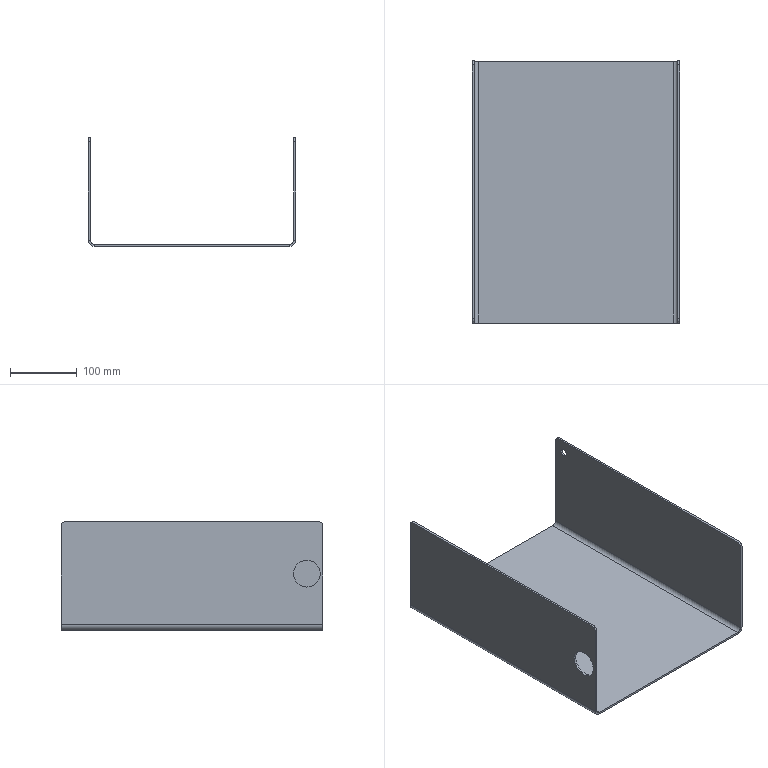Part | SolidWorks | features Cut 2, FlatPattern 1, ICE 1, SMBaseFlange 1, SheetMetal 1 | 1 solid | 30 faces | box 310 x 391 x 162 mm | volume 724944 mm3 | plane 18 | cylinder 12 | commonest cylinder face diameters 12 x6 11 x2 18 x2 40 x2
STEP:
#1=CARTESIAN_POINT('',(0.,24.,-97.5));
#2=VERTEX_POINT('',#1);
#3=CARTESIAN_POINT('',(0.,24.,-57.5));
#4=VERTEX_POINT('',#3);
#5=CARTESIAN_POINT('',(0.,24.,-77.5));
#6=DIRECTION('',(-1.,0.,0.));
#7=DIRECTION('',(0.,0.,1.));
#8=AXIS2_PLACEMENT_3D('',#5,#6,#7);
#9=CIRCLE('',#8,20.);
#10=EDGE_CURVE('',#2,#4,#9,.T.);
#11=ORIENTED_EDGE('',*,*,#10,.F.);
#12=CARTESIAN_POINT('',(-3.,24.,-97.5));
#13=VERTEX_POINT('',#12);
#14=CARTESIAN_POINT('',(7.,24.,-97.5));
#15=DIRECTION('',(-1.,0.,0.));
#16=VECTOR('',#15,1000.);
#17=LINE('',#14,#16);
#18=EDGE_CURVE('',#2,#13,#17,.T.);
#19=ORIENTED_EDGE('',*,*,#18,.T.);
#20=CARTESIAN_POINT('',(-3.,24.,-57.5));
#21=VERTEX_POINT('',#20);
#22=CARTESIAN_POINT('',(-3.,24.,-77.5));
#23=DIRECTION('',(-1.,0.,0.));
#24=DIRECTION('',(0.,0.,1.));
#25=AXIS2_PLACEMENT_3D('',#22,#23,#24);
#26=CIRCLE('',#25,20.);
#27=EDGE_CURVE('',#13,#21,#26,.T.);
#28=ORIENTED_EDGE('',*,*,#27,.T.);
#29=CARTESIAN_POINT('',(7.,24.,-57.5));
#30=DIRECTION('',(-1.,0.,0.));
#31=VECTOR('',#30,1000.);
#32=LINE('',#29,#31);
#33=EDGE_CURVE('',#4,#21,#32,.T.);
#34=ORIENTED_EDGE('',*,*,#33,.F.);
#35=EDGE_LOOP('',(#11,#19,#28,#34));
#36=FACE_OUTER_BOUND('',#35,.T.);
#37=CARTESIAN_POINT('',(7.,24.,-77.5));
#38=DIRECTION('',(-1.,0.,0.));
#39=DIRECTION('',(0.,0.,1.));
#40=AXIS2_PLACEMENT_3D('',#37,#38,#39);
#41=CYLINDRICAL_SURFACE('',#40,20.);
#42=ADVANCED_FACE('',(#36),#41,.F.);
#43=CARTESIAN_POINT('',(304.,374.,-14.5));
#44=VERTEX_POINT('',#43);
#45=CARTESIAN_POINT('',(304.,374.,-25.5));
#46=VERTEX_POINT('',#45);
#47=CARTESIAN_POINT('',(304.,374.,-20.));
#48=DIRECTION('',(1.,0.,0.));
#49=DIRECTION('',(0.,0.,-1.));
#50=AXIS2_PLACEMENT_3D('',#47,#48,#49);
#51=CIRCLE('',#50,5.5);
#52=EDGE_CURVE('',#44,#46,#51,.T.);
#53=ORIENTED_EDGE('',*,*,#52,.F.);
#54=CARTESIAN_POINT('',(307.,374.,-14.5));
#55=VERTEX_POINT('',#54);
#56=CARTESIAN_POINT('',(297.,374.,-14.5));
#57=DIRECTION('',(1.,0.,0.));
#58=VECTOR('',#57,1000.);
#59=LINE('',#56,#58);
#60=EDGE_CURVE('',#44,#55,#59,.T.);
#61=ORIENTED_EDGE('',*,*,#60,.T.);
#62=CARTESIAN_POINT('',(307.,374.,-25.5));
#63=VERTEX_POINT('',#62);
#64=CARTESIAN_POINT('',(307.,374.,-20.));
#65=DIRECTION('',(1.,0.,0.));
#66=DIRECTION('',(0.,0.,-1.));
#67=AXIS2_PLACEMENT_3D('',#64,#65,#66);
#68=CIRCLE('',#67,5.5);
#69=EDGE_CURVE('',#55,#63,#68,.T.);
#70=ORIENTED_EDGE('',*,*,#69,.T.);
#71=CARTESIAN_POINT('',(297.,374.,-25.5));
#72=DIRECTION('',(1.,0.,0.));
#73=VECTOR('',#72,1000.);
#74=LINE('',#71,#73);
#75=EDGE_CURVE('',#46,#63,#74,.T.);
#76=ORIENTED_EDGE('',*,*,#75,.F.);
#77=EDGE_LOOP('',(#53,#61,#70,#76));
#78=FACE_OUTER_BOUND('',#77,.T.);
#79=CARTESIAN_POINT('',(297.,374.,-20.));
#80=DIRECTION('',(1.,0.,0.));
#81=DIRECTION('',(0.,0.,-1.));
#82=AXIS2_PLACEMENT_3D('',#79,#80,#81);
#83=CYLINDRICAL_SURFACE('',#82,5.5);
#84=ADVANCED_FACE('',(#78),#83,.F.);
#85=CARTESIAN_POINT('',(304.,374.,-20.));
#86=DIRECTION('',(1.,0.,0.));
#87=DIRECTION('',(0.,0.,-1.));
#88=AXIS2_PLACEMENT_3D('',#85,#86,#87);
#89=CIRCLE('',#88,5.5);
#90=EDGE_CURVE('',#46,#44,#89,.T.);
#91=ORIENTED_EDGE('',*,*,#90,.T.);
#92=ORIENTED_EDGE('',*,*,#52,.T.);
#93=EDGE_LOOP('',(#91,#92));
#94=FACE_BOUND('',#93,.T.);
#95=CARTESIAN_POINT('',(304.,0.,-6.));
#96=VERTEX_POINT('',#95);
#97=CARTESIAN_POINT('',(304.,6.,0.));
#98=VERTEX_POINT('',#97);
#99=CARTESIAN_POINT('',(304.,6.,-6.));
#100=DIRECTION('',(-1.,0.,0.));
#101=DIRECTION('',(0.,0.,-1.));
#102=AXIS2_PLACEMENT_3D('',#99,#100,#101);
#103=CIRCLE('',#102,6.);
#104=EDGE_CURVE('',#96,#98,#103,.T.);
#105=ORIENTED_EDGE('',*,*,#104,.T.);
#106=CARTESIAN_POINT('',(304.,385.,0.));
#107=VERTEX_POINT('',#106);
#108=CARTESIAN_POINT('',(304.,391.,0.));
#109=DIRECTION('',(0.,-1.,0.));
#110=VECTOR('',#109,1000.);
#111=LINE('',#108,#110);
#112=EDGE_CURVE('',#107,#98,#111,.T.);
#113=ORIENTED_EDGE('',*,*,#112,.F.);
#114=CARTESIAN_POINT('',(304.,391.,-6.));
#115=VERTEX_POINT('',#114);
#116=CARTESIAN_POINT('',(304.,385.,-6.));
#117=DIRECTION('',(-1.,0.,0.));
#118=DIRECTION('',(0.,0.,-1.));
#119=AXIS2_PLACEMENT_3D('',#116,#117,#118);
#120=CIRCLE('',#119,6.);
#121=EDGE_CURVE('',#107,#115,#120,.T.);
#122=ORIENTED_EDGE('',*,*,#121,.T.);
#123=CARTESIAN_POINT('',(304.,391.,-153.));
#124=VERTEX_POINT('',#123);
#125=CARTESIAN_POINT('',(304.,391.,-153.));
#126=DIRECTION('',(0.,0.,1.));
#127=VECTOR('',#126,1000.);
#128=LINE('',#125,#127);
#129=EDGE_CURVE('',#124,#115,#128,.T.);
#130=ORIENTED_EDGE('',*,*,#129,.F.);
#131=CARTESIAN_POINT('',(304.,0.,-153.));
#132=VERTEX_POINT('',#131);
#133=CARTESIAN_POINT('',(304.,391.,-153.));
#134=DIRECTION('',(0.,-1.,0.));
#135=VECTOR('',#134,1000.);
#136=LINE('',#133,#135);
#137=EDGE_CURVE('',#124,#132,#136,.T.);
#138=ORIENTED_EDGE('',*,*,#137,.T.);
#139=CARTESIAN_POINT('',(304.,0.,-153.));
#140=DIRECTION('',(0.,0.,1.));
#141=VECTOR('',#140,1000.);
#142=LINE('',#139,#141);
#143=EDGE_CURVE('',#132,#96,#142,.T.);
#144=ORIENTED_EDGE('',*,*,#143,.T.);
#145=EDGE_LOOP('',(#105,#113,#122,#130,#138,#144));
#146=FACE_OUTER_BOUND('',#145,.T.);
#147=CARTESIAN_POINT('',(304.,391.,-153.));
#148=DIRECTION('',(1.,0.,0.));
#149=DIRECTION('',(0.,0.,-1.));
#150=AXIS2_PLACEMENT_3D('',#147,#148,#149);
#151=PLANE('',#150);
#152=ADVANCED_FACE('',(#94,#146),#151,.F.);
#153=CARTESIAN_POINT('',(307.,374.,-20.));
#154=DIRECTION('',(1.,0.,0.));
#155=DIRECTION('',(0.,0.,-1.));
#156=AXIS2_PLACEMENT_3D('',#153,#154,#155);
#157=CIRCLE('',#156,5.5);
#158=EDGE_CURVE('',#63,#55,#157,.T.);
#159=ORIENTED_EDGE('',*,*,#158,.F.);
#160=ORIENTED_EDGE('',*,*,#69,.F.);
#161=EDGE_LOOP('',(#159,#160));
#162=FACE_BOUND('',#161,.T.);
#163=CARTESIAN_POINT('',(307.,385.,0.));
#164=VERTEX_POINT('',#163);
#165=CARTESIAN_POINT('',(307.,6.,0.));
#166=VERTEX_POINT('',#165);
#167=CARTESIAN_POINT('',(307.,391.,0.));
#168=DIRECTION('',(0.,-1.,0.));
#169=VECTOR('',#168,1000.);
#170=LINE('',#167,#169);
#171=EDGE_CURVE('',#164,#166,#170,.T.);
#172=ORIENTED_EDGE('',*,*,#171,.T.);
#173=CARTESIAN_POINT('',(307.,0.,-6.));
#174=VERTEX_POINT('',#173);
#175=CARTESIAN_POINT('',(307.,6.,-6.));
#176=DIRECTION('',(-1.,0.,0.));
#177=DIRECTION('',(0.,0.,-1.));
#178=AXIS2_PLACEMENT_3D('',#175,#176,#177);
#179=CIRCLE('',#178,6.);
#180=EDGE_CURVE('',#174,#166,#179,.T.);
#181=ORIENTED_EDGE('',*,*,#180,.F.);
#182=CARTESIAN_POINT('',(307.,0.,-153.));
#183=VERTEX_POINT('',#182);
#184=CARTESIAN_POINT('',(307.,0.,-153.));
#185=DIRECTION('',(0.,0.,1.));
#186=VECTOR('',#185,1000.);
#187=LINE('',#184,#186);
#188=EDGE_CURVE('',#183,#174,#187,.T.);
#189=ORIENTED_EDGE('',*,*,#188,.F.);
#190=CARTESIAN_POINT('',(307.,391.,-153.));
#191=VERTEX_POINT('',#190);
#192=CARTESIAN_POINT('',(307.,391.,-153.));
#193=DIRECTION('',(0.,-1.,0.));
#194=VECTOR('',#193,1000.);
#195=LINE('',#192,#194);
#196=EDGE_CURVE('',#191,#183,#195,.T.);
#197=ORIENTED_EDGE('',*,*,#196,.F.);
#198=CARTESIAN_POINT('',(307.,391.,-6.));
#199=VERTEX_POINT('',#198);
#200=CARTESIAN_POINT('',(307.,391.,-153.));
#201=DIRECTION('',(0.,0.,1.));
#202=VECTOR('',#201,1000.);
#203=LINE('',#200,#202);
#204=EDGE_CURVE('',#191,#199,#203,.T.);
#205=ORIENTED_EDGE('',*,*,#204,.T.);
#206=CARTESIAN_POINT('',(307.,385.,-6.));
#207=DIRECTION('',(-1.,0.,0.));
#208=DIRECTION('',(0.,0.,-1.));
#209=AXIS2_PLACEMENT_3D('',#206,#207,#208);
#210=CIRCLE('',#209,6.);
#211=EDGE_CURVE('',#164,#199,#210,.T.);
#212=ORIENTED_EDGE('',*,*,#211,.F.);
#213=EDGE_LOOP('',(#172,#181,#189,#197,#205,#212));
#214=FACE_OUTER_BOUND('',#213,.T.);
#215=CARTESIAN_POINT('',(307.,391.,-153.));
#216=DIRECTION('',(1.,0.,0.));
#217=DIRECTION('',(0.,0.,-1.));
#218=AXIS2_PLACEMENT_3D('',#215,#216,#217);
#219=PLANE('',#218);
#220=ADVANCED_FACE('',(#162,#214),#219,.T.);
#221=ORIENTED_EDGE('',*,*,#112,.T.);
#222=CARTESIAN_POINT('',(304.,6.,0.));
#223=DIRECTION('',(1.,0.,0.));
#224=VECTOR('',#223,1000.);
#225=LINE('',#222,#224);
#226=EDGE_CURVE('',#98,#166,#225,.T.);
#227=ORIENTED_EDGE('',*,*,#226,.T.);
#228=ORIENTED_EDGE('',*,*,#171,.F.);
#229=CARTESIAN_POINT('',(304.,385.,0.));
#230=DIRECTION('',(1.,0.,0.));
#231=VECTOR('',#230,1000.);
#232=LINE('',#229,#231);
#233=EDGE_CURVE('',#107,#164,#232,.T.);
#234=ORIENTED_EDGE('',*,*,#233,.F.);
#235=EDGE_LOOP('',(#221,#227,#228,#234));
#236=FACE_OUTER_BOUND('',#235,.T.);
#237=CARTESIAN_POINT('',(307.,391.,0.));
#238=DIRECTION('',(0.,0.,1.));
#239=DIRECTION('',(1.,0.,0.));
#240=AXIS2_PLACEMENT_3D('',#237,#238,#239);
#241=PLANE('',#240);
#242=ADVANCED_FACE('',(#236),#241,.T.);
#243=CARTESIAN_POINT('',(-3.,24.,-77.5));
#244=DIRECTION('',(-1.,0.,0.));
#245=DIRECTION('',(0.,0.,1.));
#246=AXIS2_PLACEMENT_3D('',#243,#244,#245);
#247=CIRCLE('',#246,20.);
#248=EDGE_CURVE('',#21,#13,#247,.T.);
#249=ORIENTED_EDGE('',*,*,#248,.F.);
#250=ORIENTED_EDGE('',*,*,#27,.F.);
#251=EDGE_LOOP('',(#249,#250));
#252=FACE_BOUND('',#251,.T.);
#253=CARTESIAN_POINT('',(-3.,0.,-6.));
#254=VERTEX_POINT('',#253);
#255=CARTESIAN_POINT('',(-3.,0.,-153.));
#256=VERTEX_POINT('',#255);
#257=CARTESIAN_POINT('',(-3.,0.,0.));
#258=DIRECTION('',(0.,0.,-1.));
#259=VECTOR('',#258,1000.);
#260=LINE('',#257,#259);
#261=EDGE_CURVE('',#254,#256,#260,.T.);
#262=ORIENTED_EDGE('',*,*,#261,.F.);
#263=CARTESIAN_POINT('',(-3.,6.,0.));
#264=VERTEX_POINT('',#263);
#265=CARTESIAN_POINT('',(-3.,6.,-6.));
#266=DIRECTION('',(1.,0.,0.));
#267=DIRECTION('',(0.,0.,1.));
#268=AXIS2_PLACEMENT_3D('',#265,#266,#267);
#269=CIRCLE('',#268,6.);
#270=EDGE_CURVE('',#264,#254,#269,.T.);
#271=ORIENTED_EDGE('',*,*,#270,.F.);
#272=CARTESIAN_POINT('',(-3.,385.,0.));
#273=VERTEX_POINT('',#272);
#274=CARTESIAN_POINT('',(-3.,391.,0.));
#275=DIRECTION('',(0.,-1.,0.));
#276=VECTOR('',#275,1000.);
#277=LINE('',#274,#276);
#278=EDGE_CURVE('',#273,#264,#277,.T.);
#279=ORIENTED_EDGE('',*,*,#278,.F.);
#280=CARTESIAN_POINT('',(-3.,391.,-6.));
#281=VERTEX_POINT('',#280);
#282=CARTESIAN_POINT('',(-3.,385.,-6.));
#283=DIRECTION('',(1.,0.,0.));
#284=DIRECTION('',(0.,0.,1.));
#285=AXIS2_PLACEMENT_3D('',#282,#283,#284);
#286=CIRCLE('',#285,6.);
#287=EDGE_CURVE('',#281,#273,#286,.T.);
#288=ORIENTED_EDGE('',*,*,#287,.F.);
#289=CARTESIAN_POINT('',(-3.,391.,-153.));
#290=VERTEX_POINT('',#289);
#291=CARTESIAN_POINT('',(-3.,391.,0.));
#292=DIRECTION('',(0.,0.,-1.));
#293=VECTOR('',#292,1000.);
#294=LINE('',#291,#293);
#295=EDGE_CURVE('',#281,#290,#294,.T.);
#296=ORIENTED_EDGE('',*,*,#295,.T.);
#297=CARTESIAN_POINT('',(-3.,391.,-153.));
#298=DIRECTION('',(0.,-1.,0.));
#299=VECTOR('',#298,1000.);
#300=LINE('',#297,#299);
#301=EDGE_CURVE('',#290,#256,#300,.T.);
#302=ORIENTED_EDGE('',*,*,#301,.T.);
#303=EDGE_LOOP('',(#262,#271,#279,#288,#296,#302));
#304=FACE_OUTER_BOUND('',#303,.T.);
#305=CARTESIAN_POINT('',(-3.,391.,0.));
#306=DIRECTION('',(-1.,0.,0.));
#307=DIRECTION('',(0.,0.,1.));
#308=AXIS2_PLACEMENT_3D('',#305,#306,#307);
#309=PLANE('',#308);
#310=ADVANCED_FACE('',(#252,#304),#309,.T.);
#311=CARTESIAN_POINT('',(0.,24.,-77.5));
#312=DIRECTION('',(-1.,0.,0.));
#313=DIRECTION('',(0.,0.,1.));
#314=AXIS2_PLACEMENT_3D('',#311,#312,#313);
#315=CIRCLE('',#314,20.);
#316=EDGE_CURVE('',#4,#2,#315,.T.);
#317=ORIENTED_EDGE('',*,*,#316,.T.);
#318=ORIENTED_EDGE('',*,*,#10,.T.);
#319=EDGE_LOOP('',(#317,#318));
#320=FACE_BOUND('',#319,.T.);
#321=CARTESIAN_POINT('',(0.,6.,0.));
#322=VERTEX_POINT('',#321);
#323=CARTESIAN_POINT('',(0.,0.,-6.));
#324=VERTEX_POINT('',#323);
#325=CARTESIAN_POINT('',(0.,6.,-6.));
#326=DIRECTION('',(1.,0.,0.));
#327=DIRECTION('',(0.,0.,1.));
#328=AXIS2_PLACEMENT_3D('',#325,#326,#327);
#329=CIRCLE('',#328,6.);
#330=EDGE_CURVE('',#322,#324,#329,.T.);
#331=ORIENTED_EDGE('',*,*,#330,.T.);
#332=CARTESIAN_POINT('',(0.,0.,-153.));
#333=VERTEX_POINT('',#332);
#334=CARTESIAN_POINT('',(0.,0.,0.));
#335=DIRECTION('',(0.,0.,-1.));
#336=VECTOR('',#335,1000.);
#337=LINE('',#334,#336);
#338=EDGE_CURVE('',#324,#333,#337,.T.);
#339=ORIENTED_EDGE('',*,*,#338,.T.);
#340=CARTESIAN_POINT('',(0.,391.,-153.));
#341=VERTEX_POINT('',#340);
#342=CARTESIAN_POINT('',(0.,391.,-153.));
#343=DIRECTION('',(0.,-1.,0.));
#344=VECTOR('',#343,1000.);
#345=LINE('',#342,#344);
#346=EDGE_CURVE('',#341,#333,#345,.T.);
#347=ORIENTED_EDGE('',*,*,#346,.F.);
#348=CARTESIAN_POINT('',(0.,391.,-6.));
#349=VERTEX_POINT('',#348);
#350=CARTESIAN_POINT('',(0.,391.,0.));
#351=DIRECTION('',(0.,0.,-1.));
#352=VECTOR('',#351,1000.);
#353=LINE('',#350,#352);
#354=EDGE_CURVE('',#349,#341,#353,.T.);
#355=ORIENTED_EDGE('',*,*,#354,.F.);
#356=CARTESIAN_POINT('',(0.,385.,0.));
#357=VERTEX_POINT('',#356);
#358=CARTESIAN_POINT('',(0.,385.,-6.));
#359=DIRECTION('',(1.,0.,0.));
#360=DIRECTION('',(0.,0.,1.));
#361=AXIS2_PLACEMENT_3D('',#358,#359,#360);
#362=CIRCLE('',#361,6.);
#363=EDGE_CURVE('',#349,#357,#362,.T.);
#364=ORIENTED_EDGE('',*,*,#363,.T.);
#365=CARTESIAN_POINT('',(0.,391.,0.));
#366=DIRECTION('',(0.,-1.,0.));
#367=VECTOR('',#366,1000.);
#368=LINE('',#365,#367);
#369=EDGE_CURVE('',#357,#322,#368,.T.);
#370=ORIENTED_EDGE('',*,*,#369,.T.);
#371=EDGE_LOOP('',(#331,#339,#347,#355,#364,#370));
#372=FACE_OUTER_BOUND('',#371,.T.);
#373=CARTESIAN_POINT('',(0.,391.,0.));
#374=DIRECTION('',(-1.,0.,0.));
#375=DIRECTION('',(0.,0.,1.));
#376=AXIS2_PLACEMENT_3D('',#373,#374,#375);
#377=PLANE('',#376);
#378=ADVANCED_FACE('',(#320,#372),#377,.F.);
#379=ORIENTED_EDGE('',*,*,#129,.T.);
#380=CARTESIAN_POINT('',(304.,391.,-6.));
#381=DIRECTION('',(1.,0.,0.));
#382=VECTOR('',#381,1000.);
#383=LINE('',#380,#382);
#384=EDGE_CURVE('',#115,#199,#383,.T.);
#385=ORIENTED_EDGE('',*,*,#384,.T.);
#386=ORIENTED_EDGE('',*,*,#204,.F.);
#387=CARTESIAN_POINT('',(307.,391.,-153.));
#388=DIRECTION('',(-1.,0.,0.));
#389=VECTOR('',#388,1000.);
#390=LINE('',#387,#389);
#391=EDGE_CURVE('',#191,#124,#390,.T.);
#392=ORIENTED_EDGE('',*,*,#391,.T.);
#393=EDGE_LOOP('',(#379,#385,#386,#392));
#394=FACE_OUTER_BOUND('',#393,.T.);
#395=CARTESIAN_POINT('',(298.,391.,-153.));
#396=DIRECTION('',(0.,1.,0.));
#397=DIRECTION('',(1.,0.,0.));
#398=AXIS2_PLACEMENT_3D('',#395,#396,#397);
#399=PLANE('',#398);
#400=ADVANCED_FACE('',(#394),#399,.T.);
#401=CARTESIAN_POINT('',(0.,6.,0.));
#402=DIRECTION('',(-1.,0.,0.));
#403=VECTOR('',#402,1000.);
#404=LINE('',#401,#403);
#405=EDGE_CURVE('',#322,#264,#404,.T.);
#406=ORIENTED_EDGE('',*,*,#405,.F.);
#407=ORIENTED_EDGE('',*,*,#369,.F.);
#408=CARTESIAN_POINT('',(0.,385.,0.));
#409=DIRECTION('',(-1.,0.,0.));
#410=VECTOR('',#409,1000.);
#411=LINE('',#408,#410);
#412=EDGE_CURVE('',#357,#273,#411,.T.);
#413=ORIENTED_EDGE('',*,*,#412,.T.);
#414=ORIENTED_EDGE('',*,*,#278,.T.);
#415=EDGE_LOOP('',(#406,#407,#413,#414));
#416=FACE_OUTER_BOUND('',#415,.T.);
#417=CARTESIAN_POINT('',(0.,391.,0.));
#418=DIRECTION('',(0.,0.,1.));
#419=DIRECTION('',(1.,0.,0.));
#420=AXIS2_PLACEMENT_3D('',#417,#418,#419);
#421=PLANE('',#420);
#422=ADVANCED_FACE('',(#416),#421,.T.);
#423=CARTESIAN_POINT('',(0.,391.,-153.));
#424=DIRECTION('',(-1.,0.,0.));
#425=VECTOR('',#424,1000.);
#426=LINE('',#423,#425);
#427=EDGE_CURVE('',#341,#290,#426,.T.);
#428=ORIENTED_EDGE('',*,*,#427,.F.);
#429=CARTESIAN_POINT('',(6.,391.,-159.));
#430=VERTEX_POINT('',#429);
#431=CARTESIAN_POINT('',(6.,391.,-153.));
#432=DIRECTION('',(0.,-1.,0.));
#433=DIRECTION('',(0.,0.,1.));
#434=AXIS2_PLACEMENT_3D('',#431,#432,#433);
#435=CIRCLE('',#434,6.);
#436=EDGE_CURVE('',#341,#430,#435,.T.);
#437=ORIENTED_EDGE('',*,*,#436,.T.);
#438=CARTESIAN_POINT('',(6.,391.,-162.));
#439=VERTEX_POINT('',#438);
#440=CARTESIAN_POINT('',(6.,391.,-162.));
#441=DIRECTION('',(0.,0.,1.));
#442=VECTOR('',#441,1000.);
#443=LINE('',#440,#442);
#444=EDGE_CURVE('',#439,#430,#443,.T.);
#445=ORIENTED_EDGE('',*,*,#444,.F.);
#446=CARTESIAN_POINT('',(6.,391.,-153.));
#447=DIRECTION('',(0.,-1.,0.));
#448=DIRECTION('',(1.,0.,0.));
#449=AXIS2_PLACEMENT_3D('',#446,#447,#448);
#450=CIRCLE('',#449,9.);
#451=EDGE_CURVE('',#290,#439,#450,.T.);
#452=ORIENTED_EDGE('',*,*,#451,.F.);
#453=EDGE_LOOP('',(#428,#437,#445,#452));
#454=FACE_OUTER_BOUND('',#453,.T.);
#455=CARTESIAN_POINT('',(0.,391.,-153.));
#456=DIRECTION('',(0.,1.,0.));
#457=DIRECTION('',(0.,0.,1.));
#458=AXIS2_PLACEMENT_3D('',#455,#456,#457);
#459=PLANE('',#458);
#460=ADVANCED_FACE('',(#454),#459,.T.);
#461=CARTESIAN_POINT('',(0.,391.,-6.));
#462=DIRECTION('',(-1.,0.,0.));
#463=VECTOR('',#462,1000.);
#464=LINE('',#461,#463);
#465=EDGE_CURVE('',#349,#281,#464,.T.);
#466=ORIENTED_EDGE('',*,*,#465,.F.);
#467=ORIENTED_EDGE('',*,*,#354,.T.);
#468=ORIENTED_EDGE('',*,*,#427,.T.);
#469=ORIENTED_EDGE('',*,*,#295,.F.);
#470=EDGE_LOOP('',(#466,#467,#468,#469));
#471=FACE_OUTER_BOUND('',#470,.T.);
#472=CARTESIAN_POINT('',(6.,391.,-162.));
#473=DIRECTION('',(0.,1.,0.));
#474=DIRECTION('',(0.,0.,1.));
#475=AXIS2_PLACEMENT_3D('',#472,#473,#474);
#476=PLANE('',#475);
#477=ADVANCED_FACE('',(#471),#476,.T.);
#478=CARTESIAN_POINT('',(6.,0.,-159.));
#479=VERTEX_POINT('',#478);
#480=CARTESIAN_POINT('',(6.,0.,-162.));
#481=VERTEX_POINT('',#480);
#482=CARTESIAN_POINT('',(6.,0.,-159.));
#483=DIRECTION('',(0.,0.,-1.));
#484=VECTOR('',#483,1000.);
#485=LINE('',#482,#484);
#486=EDGE_CURVE('',#479,#481,#485,.T.);
#487=ORIENTED_EDGE('',*,*,#486,.F.);
#488=CARTESIAN_POINT('',(6.,0.,-153.));
#489=DIRECTION('',(0.,-1.,0.));
#490=DIRECTION('',(0.,0.,1.));
#491=AXIS2_PLACEMENT_3D('',#488,#489,#490);
#492=CIRCLE('',#491,6.);
#493=EDGE_CURVE('',#333,#479,#492,.T.);
#494=ORIENTED_EDGE('',*,*,#493,.F.);
#495=CARTESIAN_POINT('',(-3.,0.,-153.));
#496=DIRECTION('',(1.,0.,0.));
#497=VECTOR('',#496,1000.);
#498=LINE('',#495,#497);
#499=EDGE_CURVE('',#256,#333,#498,.T.);
#500=ORIENTED_EDGE('',*,*,#499,.F.);
#501=CARTESIAN_POINT('',(6.,0.,-153.));
#502=DIRECTION('',(0.,-1.,0.));
#503=DIRECTION('',(1.,0.,0.));
#504=AXIS2_PLACEMENT_3D('',#501,#502,#503);
#505=CIRCLE('',#504,9.);
#506=EDGE_CURVE('',#256,#481,#505,.T.);
#507=ORIENTED_EDGE('',*,*,#506,.T.);
#508=EDGE_LOOP('',(#487,#494,#500,#507));
#509=FACE_OUTER_BOUND('',#508,.T.);
#510=CARTESIAN_POINT('',(6.,0.,-159.));
#511=DIRECTION('',(0.,-1.,0.));
#512=DIRECTION('',(0.,0.,-1.));
#513=AXIS2_PLACEMENT_3D('',#510,#511,#512);
#514=PLANE('',#513);
#515=ADVANCED_FACE('',(#509),#514,.T.);
#516=CARTESIAN_POINT('',(298.,0.,-159.));
#517=VERTEX_POINT('',#516);
#518=CARTESIAN_POINT('',(6.,0.,-159.));
#519=DIRECTION('',(1.,0.,0.));
#520=VECTOR('',#519,1000.);
#521=LINE('',#518,#520);
#522=EDGE_CURVE('',#479,#517,#521,.T.);
#523=ORIENTED_EDGE('',*,*,#522,.F.);
#524=ORIENTED_EDGE('',*,*,#486,.T.);
#525=CARTESIAN_POINT('',(298.,0.,-162.));
#526=VERTEX_POINT('',#525);
#527=CARTESIAN_POINT('',(6.,0.,-162.));
#528=DIRECTION('',(1.,0.,0.));
#529=VECTOR('',#528,1000.);
#530=LINE('',#527,#529);
#531=EDGE_CURVE('',#481,#526,#530,.T.);
#532=ORIENTED_EDGE('',*,*,#531,.T.);
#533=CARTESIAN_POINT('',(298.,0.,-162.));
#534=DIRECTION('',(0.,0.,1.));
#535=VECTOR('',#534,1000.);
#536=LINE('',#533,#535);
#537=EDGE_CURVE('',#526,#517,#536,.T.);
#538=ORIENTED_EDGE('',*,*,#537,.T.);
#539=EDGE_LOOP('',(#523,#524,#532,#538));
#540=FACE_OUTER_BOUND('',#539,.T.);
#541=CARTESIAN_POINT('',(-3.,0.,-153.));
#542=DIRECTION('',(0.,-1.,0.));
#543=DIRECTION('',(0.,0.,-1.));
#544=AXIS2_PLACEMENT_3D('',#541,#542,#543);
#545=PLANE('',#544);
#546=ADVANCED_FACE('',(#540),#545,.T.);
#547=CARTESIAN_POINT('',(298.,391.,-159.));
#548=VERTEX_POINT('',#547);
#549=CARTESIAN_POINT('',(298.,391.,-162.));
#550=VERTEX_POINT('',#549);
#551=CARTESIAN_POINT('',(298.,391.,-159.));
#552=DIRECTION('',(0.,0.,-1.));
#553=VECTOR('',#552,1000.);
#554=LINE('',#551,#553);
#555=EDGE_CURVE('',#548,#550,#554,.T.);
#556=ORIENTED_EDGE('',*,*,#555,.F.);
#557=CARTESIAN_POINT('',(298.,391.,-153.));
#558=DIRECTION('',(0.,-1.,0.));
#559=DIRECTION('',(0.,0.,-1.));
#560=AXIS2_PLACEMENT_3D('',#557,#558,#559);
#561=CIRCLE('',#560,6.);
#562=EDGE_CURVE('',#548,#124,#561,.T.);
#563=ORIENTED_EDGE('',*,*,#562,.T.);
#564=ORIENTED_EDGE('',*,*,#391,.F.);
#565=CARTESIAN_POINT('',(298.,391.,-153.));
#566=DIRECTION('',(0.,-1.,0.));
#567=DIRECTION('',(1.,0.,0.));
#568=AXIS2_PLACEMENT_3D('',#565,#566,#567);
#569=CIRCLE('',#568,9.);
#570=EDGE_CURVE('',#550,#191,#569,.T.);
#571=ORIENTED_EDGE('',*,*,#570,.F.);
#572=EDGE_LOOP('',(#556,#563,#564,#571));
#573=FACE_OUTER_BOUND('',#572,.T.);
#574=CARTESIAN_POINT('',(298.,391.,-159.));
#575=DIRECTION('',(0.,1.,0.));
#576=DIRECTION('',(0.,0.,1.));
#577=AXIS2_PLACEMENT_3D('',#574,#575,#576);
#578=PLANE('',#577);
#579=ADVANCED_FACE('',(#573),#578,.T.);
#580=CARTESIAN_POINT('',(6.,391.,-159.));
#581=DIRECTION('',(1.,0.,0.));
#582=VECTOR('',#581,1000.);
#583=LINE('',#580,#582);
#584=EDGE_CURVE('',#430,#548,#583,.T.);
#585=ORIENTED_EDGE('',*,*,#584,.T.);
#586=ORIENTED_EDGE('',*,*,#555,.T.);
#587=CARTESIAN_POINT('',(6.,391.,-162.));
#588=DIRECTION('',(1.,0.,0.));
#589=VECTOR('',#588,1000.);
#590=LINE('',#587,#589);
#591=EDGE_CURVE('',#439,#550,#590,.T.);
#592=ORIENTED_EDGE('',*,*,#591,.F.);
#593=ORIENTED_EDGE('',*,*,#444,.T.);
#594=EDGE_LOOP('',(#585,#586,#592,#593));
#595=FACE_OUTER_BOUND('',#594,.T.);
#596=CARTESIAN_POINT('',(307.,391.,-153.));
#597=DIRECTION('',(0.,1.,0.));
#598=DIRECTION('',(0.,0.,1.));
#599=AXIS2_PLACEMENT_3D('',#596,#597,#598);
#600=PLANE('',#599);
#601=ADVANCED_FACE('',(#595),#600,.T.);
#602=CARTESIAN_POINT('',(304.,0.,-153.));
#603=DIRECTION('',(1.,0.,0.));
#604=VECTOR('',#603,1000.);
#605=LINE('',#602,#604);
#606=EDGE_CURVE('',#132,#183,#605,.T.);
#607=ORIENTED_EDGE('',*,*,#606,.F.);
#608=CARTESIAN_POINT('',(298.,0.,-153.));
#609=DIRECTION('',(0.,-1.,0.));
#610=DIRECTION('',(0.,0.,-1.));
#611=AXIS2_PLACEMENT_3D('',#608,#609,#610);
#612=CIRCLE('',#611,6.);
#613=EDGE_CURVE('',#517,#132,#612,.T.);
#614=ORIENTED_EDGE('',*,*,#613,.F.);
#615=ORIENTED_EDGE('',*,*,#537,.F.);
#616=CARTESIAN_POINT('',(298.,0.,-153.));
#617=DIRECTION('',(0.,-1.,0.));
#618=DIRECTION('',(1.,0.,0.));
#619=AXIS2_PLACEMENT_3D('',#616,#617,#618);
#620=CIRCLE('',#619,9.);
#621=EDGE_CURVE('',#526,#183,#620,.T.);
#622=ORIENTED_EDGE('',*,*,#621,.T.);
#623=EDGE_LOOP('',(#607,#614,#615,#622));
#624=FACE_OUTER_BOUND('',#623,.T.);
#625=CARTESIAN_POINT('',(304.,0.,-153.));
#626=DIRECTION('',(0.,-1.,0.));
#627=DIRECTION('',(0.,0.,-1.));
#628=AXIS2_PLACEMENT_3D('',#625,#626,#627);
#629=PLANE('',#628);
#630=ADVANCED_FACE('',(#624),#629,.T.);
#631=CARTESIAN_POINT('',(304.,0.,-6.));
#632=DIRECTION('',(1.,0.,0.));
#633=VECTOR('',#632,1000.);
#634=LINE('',#631,#633);
#635=EDGE_CURVE('',#96,#174,#634,.T.);
#636=ORIENTED_EDGE('',*,*,#635,.F.);
#637=ORIENTED_EDGE('',*,*,#143,.F.);
#638=ORIENTED_EDGE('',*,*,#606,.T.);
#639=ORIENTED_EDGE('',*,*,#188,.T.);
#640=EDGE_LOOP('',(#636,#637,#638,#639));
#641=FACE_OUTER_BOUND('',#640,.T.);
#642=CARTESIAN_POINT('',(298.,0.,-162.));
#643=DIRECTION('',(0.,-1.,0.));
#644=DIRECTION('',(0.,0.,-1.));
#645=AXIS2_PLACEMENT_3D('',#642,#643,#644);
#646=PLANE('',#645);
#647=ADVANCED_FACE('',(#641),#646,.T.);
#648=ORIENTED_EDGE('',*,*,#621,.F.);
#649=CARTESIAN_POINT('',(298.,391.,-162.));
#650=DIRECTION('',(0.,-1.,0.));
#651=VECTOR('',#650,1000.);
#652=LINE('',#649,#651);
#653=EDGE_CURVE('',#550,#526,#652,.T.);
#654=ORIENTED_EDGE('',*,*,#653,.F.);
#655=ORIENTED_EDGE('',*,*,#570,.T.);
#656=ORIENTED_EDGE('',*,*,#196,.T.);
#657=EDGE_LOOP('',(#648,#654,#655,#656));
#658=FACE_OUTER_BOUND('',#657,.T.);
#659=CARTESIAN_POINT('',(298.,391.,-153.));
#660=DIRECTION('',(0.,-1.,0.));
#661=DIRECTION('',(0.,0.,-1.));
#662=AXIS2_PLACEMENT_3D('',#659,#660,#661);
#663=CYLINDRICAL_SURFACE('',#662,9.);
#664=ADVANCED_FACE('',(#658),#663,.T.);
#665=ORIENTED_EDGE('',*,*,#531,.F.);
#666=CARTESIAN_POINT('',(6.,391.,-162.));
#667=DIRECTION('',(0.,-1.,0.));
#668=VECTOR('',#667,1000.);
#669=LINE('',#666,#668);
#670=EDGE_CURVE('',#439,#481,#669,.T.);
#671=ORIENTED_EDGE('',*,*,#670,.F.);
#672=ORIENTED_EDGE('',*,*,#591,.T.);
#673=ORIENTED_EDGE('',*,*,#653,.T.);
#674=EDGE_LOOP('',(#665,#671,#672,#673));
#675=FACE_OUTER_BOUND('',#674,.T.);
#676=CARTESIAN_POINT('',(6.,391.,-162.));
#677=DIRECTION('',(0.,0.,-1.));
#678=DIRECTION('',(-1.,0.,0.));
#679=AXIS2_PLACEMENT_3D('',#676,#677,#678);
#680=PLANE('',#679);
#681=ADVANCED_FACE('',(#675),#680,.T.);
#682=ORIENTED_EDGE('',*,*,#506,.F.);
#683=ORIENTED_EDGE('',*,*,#301,.F.);
#684=ORIENTED_EDGE('',*,*,#451,.T.);
#685=ORIENTED_EDGE('',*,*,#670,.T.);
#686=EDGE_LOOP('',(#682,#683,#684,#685));
#687=FACE_OUTER_BOUND('',#686,.T.);
#688=CARTESIAN_POINT('',(6.,391.,-153.));
#689=DIRECTION('',(0.,-1.,0.));
#690=DIRECTION('',(0.,0.,-1.));
#691=AXIS2_PLACEMENT_3D('',#688,#689,#690);
#692=CYLINDRICAL_SURFACE('',#691,9.);
#693=ADVANCED_FACE('',(#687),#692,.T.);
#694=ORIENTED_EDGE('',*,*,#493,.T.);
#695=CARTESIAN_POINT('',(6.,391.,-159.));
#696=DIRECTION('',(0.,-1.,0.));
#697=VECTOR('',#696,1000.);
#698=LINE('',#695,#697);
#699=EDGE_CURVE('',#430,#479,#698,.T.);
#700=ORIENTED_EDGE('',*,*,#699,.F.);
#701=ORIENTED_EDGE('',*,*,#436,.F.);
#702=ORIENTED_EDGE('',*,*,#346,.T.);
#703=EDGE_LOOP('',(#694,#700,#701,#702));
#704=FACE_OUTER_BOUND('',#703,.T.);
#705=CARTESIAN_POINT('',(6.,391.,-153.));
#706=DIRECTION('',(0.,-1.,0.));
#707=DIRECTION('',(0.,0.,-1.));
#708=AXIS2_PLACEMENT_3D('',#705,#706,#707);
#709=CYLINDRICAL_SURFACE('',#708,6.);
#710=ADVANCED_FACE('',(#704),#709,.F.);
#711=ORIENTED_EDGE('',*,*,#522,.T.);
#712=CARTESIAN_POINT('',(298.,391.,-159.));
#713=DIRECTION('',(0.,-1.,0.));
#714=VECTOR('',#713,1000.);
#715=LINE('',#712,#714);
#716=EDGE_CURVE('',#548,#517,#715,.T.);
#717=ORIENTED_EDGE('',*,*,#716,.F.);
#718=ORIENTED_EDGE('',*,*,#584,.F.);
#719=ORIENTED_EDGE('',*,*,#699,.T.);
#720=EDGE_LOOP('',(#711,#717,#718,#719));
#721=FACE_OUTER_BOUND('',#720,.T.);
#722=CARTESIAN_POINT('',(6.,391.,-159.));
#723=DIRECTION('',(0.,0.,-1.));
#724=DIRECTION('',(-1.,0.,0.));
#725=AXIS2_PLACEMENT_3D('',#722,#723,#724);
#726=PLANE('',#725);
#727=ADVANCED_FACE('',(#721),#726,.F.);
#728=ORIENTED_EDGE('',*,*,#613,.T.);
#729=ORIENTED_EDGE('',*,*,#137,.F.);
#730=ORIENTED_EDGE('',*,*,#562,.F.);
#731=ORIENTED_EDGE('',*,*,#716,.T.);
#732=EDGE_LOOP('',(#728,#729,#730,#731));
#733=FACE_OUTER_BOUND('',#732,.T.);
#734=CARTESIAN_POINT('',(298.,391.,-153.));
#735=DIRECTION('',(0.,-1.,0.));
#736=DIRECTION('',(0.,0.,-1.));
#737=AXIS2_PLACEMENT_3D('',#734,#735,#736);
#738=CYLINDRICAL_SURFACE('',#737,6.);
#739=ADVANCED_FACE('',(#733),#738,.F.);
#740=ORIENTED_EDGE('',*,*,#338,.F.);
#741=CARTESIAN_POINT('',(0.,0.,-6.));
#742=DIRECTION('',(-1.,0.,0.));
#743=VECTOR('',#742,1000.);
#744=LINE('',#741,#743);
#745=EDGE_CURVE('',#324,#254,#744,.T.);
#746=ORIENTED_EDGE('',*,*,#745,.T.);
#747=ORIENTED_EDGE('',*,*,#261,.T.);
#748=ORIENTED_EDGE('',*,*,#499,.T.);
#749=EDGE_LOOP('',(#740,#746,#747,#748));
#750=FACE_OUTER_BOUND('',#749,.T.);
#751=CARTESIAN_POINT('',(298.,0.,-153.));
#752=DIRECTION('',(0.,1.,0.));
#753=DIRECTION('',(1.,0.,0.));
#754=AXIS2_PLACEMENT_3D('',#751,#752,#753);
#755=PLANE('',#754);
#756=ADVANCED_FACE('',(#750),#755,.F.);
#757=ORIENTED_EDGE('',*,*,#412,.F.);
#758=ORIENTED_EDGE('',*,*,#363,.F.);
#759=ORIENTED_EDGE('',*,*,#465,.T.);
#760=ORIENTED_EDGE('',*,*,#287,.T.);
#761=EDGE_LOOP('',(#757,#758,#759,#760));
#762=FACE_OUTER_BOUND('',#761,.T.);
#763=CARTESIAN_POINT('',(0.,385.,-6.));
#764=DIRECTION('',(-1.,0.,0.));
#765=DIRECTION('',(0.,0.,1.));
#766=AXIS2_PLACEMENT_3D('',#763,#764,#765);
#767=CYLINDRICAL_SURFACE('',#766,6.);
#768=ADVANCED_FACE('',(#762),#767,.T.);
#769=ORIENTED_EDGE('',*,*,#384,.F.);
#770=ORIENTED_EDGE('',*,*,#121,.F.);
#771=ORIENTED_EDGE('',*,*,#233,.T.);
#772=ORIENTED_EDGE('',*,*,#211,.T.);
#773=EDGE_LOOP('',(#769,#770,#771,#772));
#774=FACE_OUTER_BOUND('',#773,.T.);
#775=CARTESIAN_POINT('',(304.,385.,-6.));
#776=DIRECTION('',(1.,0.,0.));
#777=DIRECTION('',(0.,0.,-1.));
#778=AXIS2_PLACEMENT_3D('',#775,#776,#777);
#779=CYLINDRICAL_SURFACE('',#778,6.);
#780=ADVANCED_FACE('',(#774),#779,.T.);
#781=ORIENTED_EDGE('',*,*,#745,.F.);
#782=ORIENTED_EDGE('',*,*,#330,.F.);
#783=ORIENTED_EDGE('',*,*,#405,.T.);
#784=ORIENTED_EDGE('',*,*,#270,.T.);
#785=EDGE_LOOP('',(#781,#782,#783,#784));
#786=FACE_OUTER_BOUND('',#785,.T.);
#787=CARTESIAN_POINT('',(0.,6.,-6.));
#788=DIRECTION('',(-1.,0.,0.));
#789=DIRECTION('',(0.,0.,1.));
#790=AXIS2_PLACEMENT_3D('',#787,#788,#789);
#791=CYLINDRICAL_SURFACE('',#790,6.);
#792=ADVANCED_FACE('',(#786),#791,.T.);
#793=ORIENTED_EDGE('',*,*,#226,.F.);
#794=ORIENTED_EDGE('',*,*,#104,.F.);
#795=ORIENTED_EDGE('',*,*,#635,.T.);
#796=ORIENTED_EDGE('',*,*,#180,.T.);
#797=EDGE_LOOP('',(#793,#794,#795,#796));
#798=FACE_OUTER_BOUND('',#797,.T.);
#799=CARTESIAN_POINT('',(304.,6.,-6.));
#800=DIRECTION('',(1.,0.,0.));
#801=DIRECTION('',(0.,0.,-1.));
#802=AXIS2_PLACEMENT_3D('',#799,#800,#801);
#803=CYLINDRICAL_SURFACE('',#802,6.);
#804=ADVANCED_FACE('',(#798),#803,.T.);
#805=ORIENTED_EDGE('',*,*,#60,.F.);
#806=ORIENTED_EDGE('',*,*,#90,.F.);
#807=ORIENTED_EDGE('',*,*,#75,.T.);
#808=ORIENTED_EDGE('',*,*,#158,.T.);
#809=EDGE_LOOP('',(#805,#806,#807,#808));
#810=FACE_OUTER_BOUND('',#809,.T.);
#811=CARTESIAN_POINT('',(297.,374.,-20.));
#812=DIRECTION('',(1.,0.,0.));
#813=DIRECTION('',(0.,0.,-1.));
#814=AXIS2_PLACEMENT_3D('',#811,#812,#813);
#815=CYLINDRICAL_SURFACE('',#814,5.5);
#816=ADVANCED_FACE('',(#810),#815,.F.);
#817=ORIENTED_EDGE('',*,*,#18,.F.);
#818=ORIENTED_EDGE('',*,*,#316,.F.);
#819=ORIENTED_EDGE('',*,*,#33,.T.);
#820=ORIENTED_EDGE('',*,*,#248,.T.);
#821=EDGE_LOOP('',(#817,#818,#819,#820));
#822=FACE_OUTER_BOUND('',#821,.T.);
#823=CARTESIAN_POINT('',(7.,24.,-77.5));
#824=DIRECTION('',(-1.,0.,0.));
#825=DIRECTION('',(0.,0.,1.));
#826=AXIS2_PLACEMENT_3D('',#823,#824,#825);
#827=CYLINDRICAL_SURFACE('',#826,20.);
#828=ADVANCED_FACE('',(#822),#827,.F.);
#829=CLOSED_SHELL('',(#42,#84,#152,#220,#242,#310,#378,#400,#422,#460,#477,#515,#546,#579,#601,#630,#647,#664,#681,#693,#710,#727,#739,#756,#768,#780,#792,#804,#816,#828));
#830=MANIFOLD_SOLID_BREP('',#829);
#831=CARTESIAN_POINT('',(0.,0.,0.));
#832=DIRECTION('',(0.,0.,1.));
#833=DIRECTION('',(1.,0.,0.));
#834=AXIS2_PLACEMENT_3D('',#831,#832,#833);
#835=(LENGTH_UNIT()NAMED_UNIT(*)SI_UNIT(.MILLI.,.METRE.));
#836=UNCERTAINTY_MEASURE_WITH_UNIT(LENGTH_MEASURE(0.00001),#835,'','');
#837=(NAMED_UNIT(*)PLANE_ANGLE_UNIT()SI_UNIT($,.RADIAN.));
#838=(NAMED_UNIT(*)SI_UNIT($,.STERADIAN.)SOLID_ANGLE_UNIT());
#839=(GEOMETRIC_REPRESENTATION_CONTEXT(3)GLOBAL_UNCERTAINTY_ASSIGNED_CONTEXT((#836))GLOBAL_UNIT_ASSIGNED_CONTEXT((#835,#837,#838))REPRESENTATION_CONTEXT('',''));
#840=ADVANCED_BREP_SHAPE_REPRESENTATION('',(#830,#834),#839);